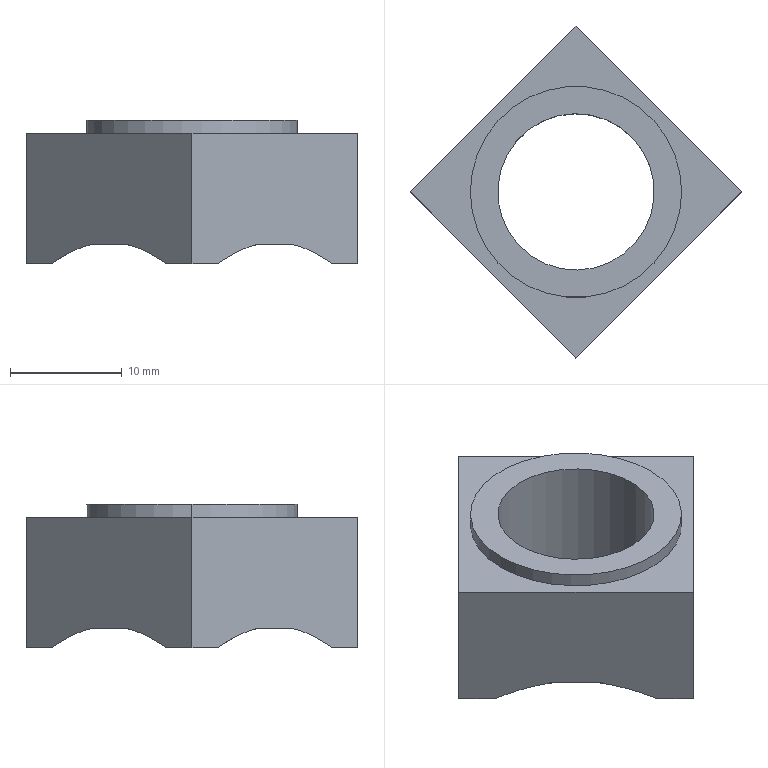Part | 1 solid | 20 faces | box 29.698 x 29.698 x 12.833 mm | volume 3074 mm3 | plane 11 | cone 5 | cylinder 4 | commonest cylinder face diameters 14 x2 18.9 x2